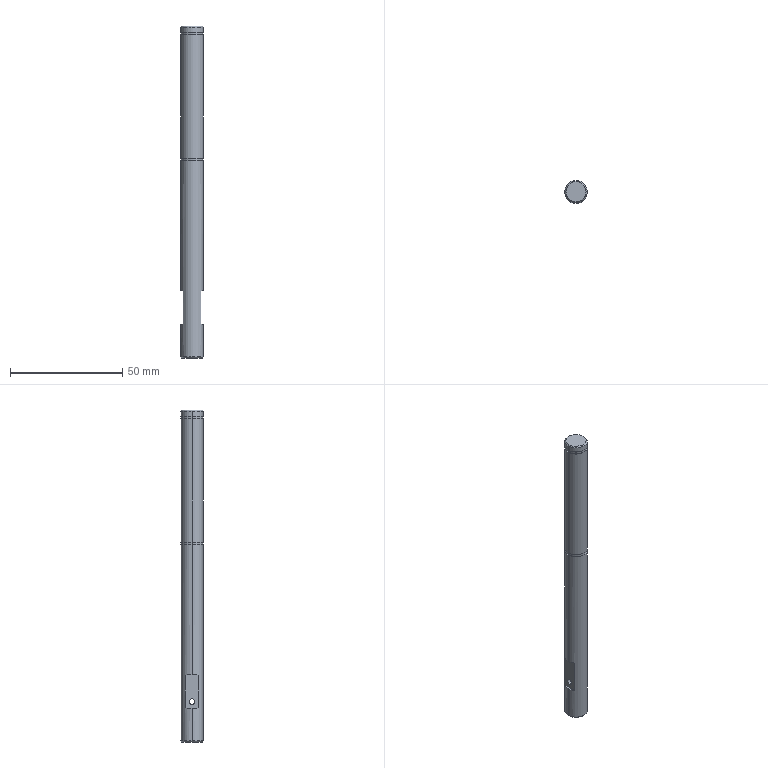Part | STEP file | 2016 Hold-down material shaft | 1 solid | 32 faces | box 10 x 10 x 148 mm | volume 11241 mm3 | cylinder 14 | plane 12 | cone 6 | commonest cylinder face diameters 10 x6 9.6 x4 2.5 x2 4.2 x2